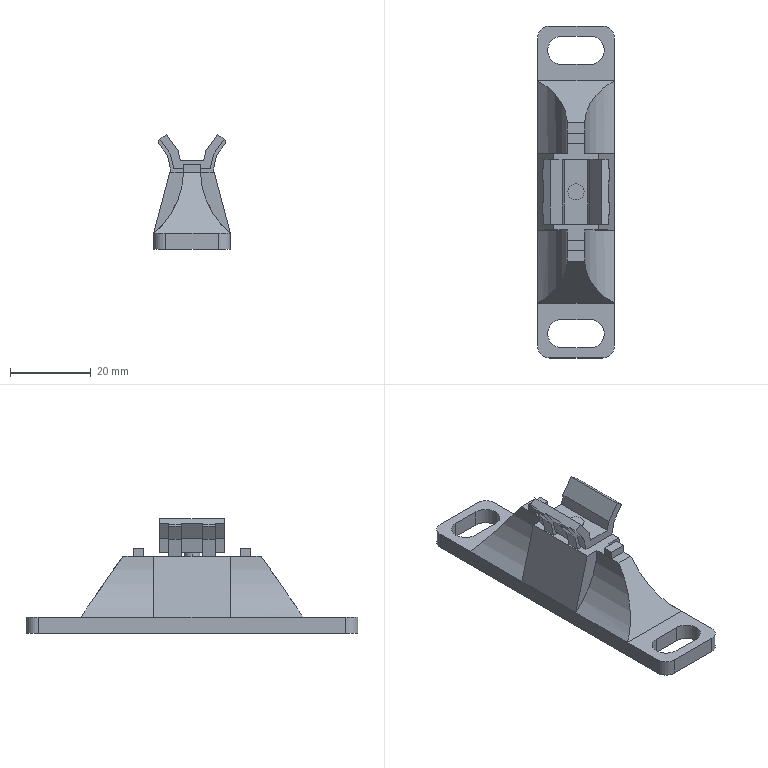Part | STEP file | 11-GY_Y300T-A_REAR-30-V10-22111.11 | 1 solid | 91 faces | box 19 x 82 x 28.4 mm | volume 14487 mm3 | plane 73 | cylinder 18 | commonest cylinder face diameters 7 x6 4 x4 6 x4 40 x4